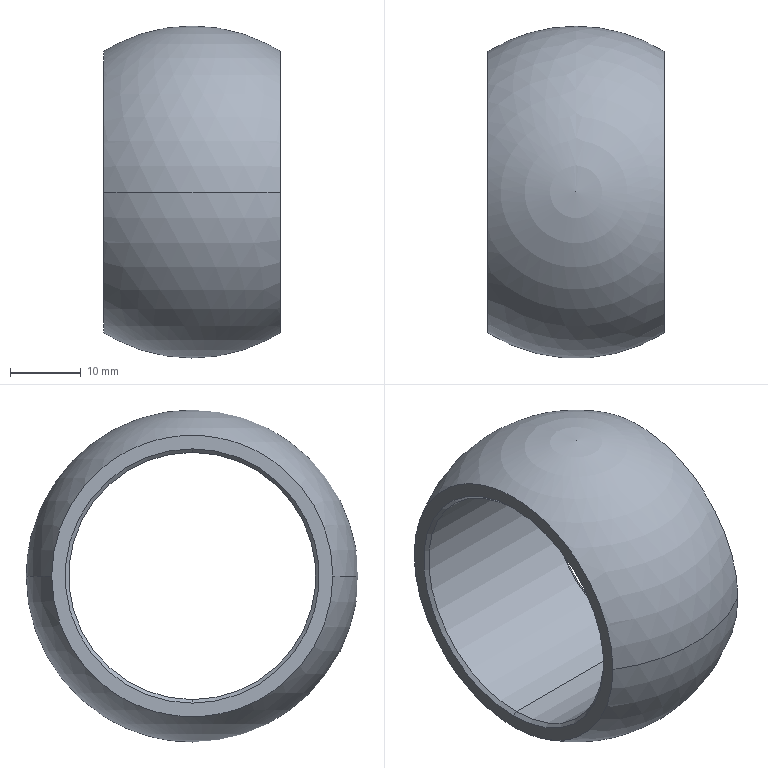Part | SolidWorks | features Chamfer 1, Revolution 1 | 1 solid | 10 faces | box 25 x 47 x 47 mm | volume 15202 mm3 | cone 4 | cylinder 2 | sphere 2 | plane 2 | commonest cylinder face diameters 35 x2
STEP:
#1=CARTESIAN_POINT('',(12.,0.,17.5));
#2=VERTEX_POINT('',#1);
#3=CARTESIAN_POINT('',(12.,0.,-17.5));
#4=VERTEX_POINT('',#3);
#5=CARTESIAN_POINT('',(12.,0.,0.));
#6=DIRECTION('',(1.,0.,0.));
#7=DIRECTION('',(0.,0.,1.));
#8=AXIS2_PLACEMENT_3D('',#5,#6,#7);
#9=CIRCLE('',#8,17.5);
#10=EDGE_CURVE('',#2,#4,#9,.T.);
#11=ORIENTED_EDGE('',*,*,#10,.F.);
#12=CARTESIAN_POINT('',(12.5,0.,18.));
#13=VERTEX_POINT('',#12);
#14=CARTESIAN_POINT('',(12.5,0.,18.));
#15=DIRECTION('',(0.7071,0.,0.7071));
#16=VECTOR('',#15,1000.);
#17=LINE('',#14,#16);
#18=EDGE_CURVE('',#2,#13,#17,.T.);
#19=ORIENTED_EDGE('',*,*,#18,.T.);
#20=CARTESIAN_POINT('',(12.5,0.,-18.));
#21=VERTEX_POINT('',#20);
#22=CARTESIAN_POINT('',(12.5,0.,0.));
#23=DIRECTION('',(-1.,0.,0.));
#24=DIRECTION('',(0.,0.,1.));
#25=AXIS2_PLACEMENT_3D('',#22,#23,#24);
#26=CIRCLE('',#25,18.);
#27=EDGE_CURVE('',#21,#13,#26,.T.);
#28=ORIENTED_EDGE('',*,*,#27,.F.);
#29=CARTESIAN_POINT('',(12.5,0.,-18.));
#30=DIRECTION('',(0.7071,0.,-0.7071));
#31=VECTOR('',#30,1000.);
#32=LINE('',#29,#31);
#33=EDGE_CURVE('',#4,#21,#32,.T.);
#34=ORIENTED_EDGE('',*,*,#33,.F.);
#35=EDGE_LOOP('',(#11,#19,#28,#34));
#36=FACE_OUTER_BOUND('',#35,.T.);
#37=CARTESIAN_POINT('',(12.5,0.,0.));
#38=DIRECTION('',(1.,0.,0.));
#39=DIRECTION('',(0.,0.,-1.));
#40=AXIS2_PLACEMENT_3D('',#37,#38,#39);
#41=CONICAL_SURFACE('',#40,18.,0.7854);
#42=ADVANCED_FACE('',(#36),#41,.F.);
#43=CARTESIAN_POINT('',(-12.,0.,-17.5));
#44=VERTEX_POINT('',#43);
#45=CARTESIAN_POINT('',(-12.,0.,17.5));
#46=VERTEX_POINT('',#45);
#47=CARTESIAN_POINT('',(-12.,0.,0.));
#48=DIRECTION('',(-1.,0.,0.));
#49=DIRECTION('',(0.,0.,-1.));
#50=AXIS2_PLACEMENT_3D('',#47,#48,#49);
#51=CIRCLE('',#50,17.5);
#52=EDGE_CURVE('',#44,#46,#51,.T.);
#53=ORIENTED_EDGE('',*,*,#52,.F.);
#54=CARTESIAN_POINT('',(-12.5,0.,-18.));
#55=VERTEX_POINT('',#54);
#56=CARTESIAN_POINT('',(-12.,0.,-17.5));
#57=DIRECTION('',(-0.7071,0.,-0.7071));
#58=VECTOR('',#57,1000.);
#59=LINE('',#56,#58);
#60=EDGE_CURVE('',#44,#55,#59,.T.);
#61=ORIENTED_EDGE('',*,*,#60,.T.);
#62=CARTESIAN_POINT('',(-12.5,0.,18.));
#63=VERTEX_POINT('',#62);
#64=CARTESIAN_POINT('',(-12.5,0.,0.));
#65=DIRECTION('',(1.,0.,0.));
#66=DIRECTION('',(0.,0.,-1.));
#67=AXIS2_PLACEMENT_3D('',#64,#65,#66);
#68=CIRCLE('',#67,18.);
#69=EDGE_CURVE('',#63,#55,#68,.T.);
#70=ORIENTED_EDGE('',*,*,#69,.F.);
#71=CARTESIAN_POINT('',(-12.,0.,17.5));
#72=DIRECTION('',(-0.7071,0.,0.7071));
#73=VECTOR('',#72,1000.);
#74=LINE('',#71,#73);
#75=EDGE_CURVE('',#46,#63,#74,.T.);
#76=ORIENTED_EDGE('',*,*,#75,.F.);
#77=EDGE_LOOP('',(#53,#61,#70,#76));
#78=FACE_OUTER_BOUND('',#77,.T.);
#79=CARTESIAN_POINT('',(-12.,0.,0.));
#80=DIRECTION('',(-1.,0.,0.));
#81=DIRECTION('',(0.,0.,1.));
#82=AXIS2_PLACEMENT_3D('',#79,#80,#81);
#83=CONICAL_SURFACE('',#82,17.5,0.7854);
#84=ADVANCED_FACE('',(#78),#83,.F.);
#85=ORIENTED_EDGE('',*,*,#10,.T.);
#86=CARTESIAN_POINT('',(-75.393,0.,-17.5));
#87=DIRECTION('',(-1.,0.,0.));
#88=VECTOR('',#87,1000.);
#89=LINE('',#86,#88);
#90=EDGE_CURVE('',#4,#44,#89,.T.);
#91=ORIENTED_EDGE('',*,*,#90,.T.);
#92=ORIENTED_EDGE('',*,*,#52,.T.);
#93=CARTESIAN_POINT('',(-75.393,0.,17.5));
#94=DIRECTION('',(-1.,0.,0.));
#95=VECTOR('',#94,1000.);
#96=LINE('',#93,#95);
#97=EDGE_CURVE('',#2,#46,#96,.T.);
#98=ORIENTED_EDGE('',*,*,#97,.F.);
#99=EDGE_LOOP('',(#85,#91,#92,#98));
#100=FACE_OUTER_BOUND('',#99,.T.);
#101=CARTESIAN_POINT('',(-75.393,0.,0.));
#102=DIRECTION('',(-1.,0.,0.));
#103=DIRECTION('',(0.,0.,1.));
#104=AXIS2_PLACEMENT_3D('',#101,#102,#103);
#105=CYLINDRICAL_SURFACE('',#104,17.5);
#106=ADVANCED_FACE('',(#100),#105,.F.);
#107=CARTESIAN_POINT('',(12.5,19.9,0.));
#108=VERTEX_POINT('',#107);
#109=CARTESIAN_POINT('',(12.5,-19.9,0.));
#110=VERTEX_POINT('',#109);
#111=CARTESIAN_POINT('',(12.5,0.,0.));
#112=DIRECTION('',(-1.,0.,0.));
#113=DIRECTION('',(0.,0.,1.));
#114=AXIS2_PLACEMENT_3D('',#111,#112,#113);
#115=CIRCLE('',#114,19.9);
#116=EDGE_CURVE('',#108,#110,#115,.T.);
#117=ORIENTED_EDGE('',*,*,#116,.T.);
#118=CARTESIAN_POINT('',(-12.5,-19.9,0.));
#119=VERTEX_POINT('',#118);
#120=CARTESIAN_POINT('',(0.,0.,0.));
#121=DIRECTION('',(0.,0.,-1.));
#122=DIRECTION('',(0.,1.,0.));
#123=AXIS2_PLACEMENT_3D('',#120,#121,#122);
#124=CIRCLE('',#123,23.5);
#125=EDGE_CURVE('',#110,#119,#124,.T.);
#126=ORIENTED_EDGE('',*,*,#125,.T.);
#127=CARTESIAN_POINT('',(-12.5,19.9,0.));
#128=VERTEX_POINT('',#127);
#129=CARTESIAN_POINT('',(-12.5,0.,0.));
#130=DIRECTION('',(-1.,0.,0.));
#131=DIRECTION('',(0.,0.,1.));
#132=AXIS2_PLACEMENT_3D('',#129,#130,#131);
#133=CIRCLE('',#132,19.9);
#134=EDGE_CURVE('',#128,#119,#133,.T.);
#135=ORIENTED_EDGE('',*,*,#134,.F.);
#136=CARTESIAN_POINT('',(0.,0.,0.));
#137=DIRECTION('',(0.,0.,1.));
#138=DIRECTION('',(1.,0.,0.));
#139=AXIS2_PLACEMENT_3D('',#136,#137,#138);
#140=CIRCLE('',#139,23.5);
#141=EDGE_CURVE('',#108,#128,#140,.T.);
#142=ORIENTED_EDGE('',*,*,#141,.F.);
#143=EDGE_LOOP('',(#117,#126,#135,#142));
#144=FACE_OUTER_BOUND('',#143,.T.);
#145=CARTESIAN_POINT('',(0.,0.,0.));
#146=DIRECTION('',(0.,0.,-1.));
#147=DIRECTION('',(0.,1.,0.));
#148=AXIS2_PLACEMENT_3D('',#145,#146,#147);
#149=SPHERICAL_SURFACE('',#148,23.5);
#150=ADVANCED_FACE('',(#144),#149,.T.);
#151=ORIENTED_EDGE('',*,*,#125,.F.);
#152=CARTESIAN_POINT('',(12.5,0.,0.));
#153=DIRECTION('',(-1.,0.,0.));
#154=DIRECTION('',(0.,0.,1.));
#155=AXIS2_PLACEMENT_3D('',#152,#153,#154);
#156=CIRCLE('',#155,19.9);
#157=EDGE_CURVE('',#110,#108,#156,.T.);
#158=ORIENTED_EDGE('',*,*,#157,.T.);
#159=ORIENTED_EDGE('',*,*,#141,.T.);
#160=CARTESIAN_POINT('',(-12.5,0.,0.));
#161=DIRECTION('',(-1.,0.,0.));
#162=DIRECTION('',(0.,0.,1.));
#163=AXIS2_PLACEMENT_3D('',#160,#161,#162);
#164=CIRCLE('',#163,19.9);
#165=EDGE_CURVE('',#119,#128,#164,.T.);
#166=ORIENTED_EDGE('',*,*,#165,.F.);
#167=EDGE_LOOP('',(#151,#158,#159,#166));
#168=FACE_OUTER_BOUND('',#167,.T.);
#169=CARTESIAN_POINT('',(0.,0.,0.));
#170=DIRECTION('',(0.,0.,-1.));
#171=DIRECTION('',(0.,1.,0.));
#172=AXIS2_PLACEMENT_3D('',#169,#170,#171);
#173=SPHERICAL_SURFACE('',#172,23.5);
#174=ADVANCED_FACE('',(#168),#173,.T.);
#175=ORIENTED_EDGE('',*,*,#69,.T.);
#176=CARTESIAN_POINT('',(-12.5,0.,0.));
#177=DIRECTION('',(1.,0.,0.));
#178=DIRECTION('',(0.,0.,-1.));
#179=AXIS2_PLACEMENT_3D('',#176,#177,#178);
#180=CIRCLE('',#179,18.);
#181=EDGE_CURVE('',#55,#63,#180,.T.);
#182=ORIENTED_EDGE('',*,*,#181,.T.);
#183=EDGE_LOOP('',(#175,#182));
#184=FACE_BOUND('',#183,.T.);
#185=ORIENTED_EDGE('',*,*,#134,.T.);
#186=ORIENTED_EDGE('',*,*,#165,.T.);
#187=EDGE_LOOP('',(#185,#186));
#188=FACE_OUTER_BOUND('',#187,.T.);
#189=CARTESIAN_POINT('',(-12.5,19.9,0.));
#190=DIRECTION('',(1.,0.,0.));
#191=DIRECTION('',(0.,0.,-1.));
#192=AXIS2_PLACEMENT_3D('',#189,#190,#191);
#193=PLANE('',#192);
#194=ADVANCED_FACE('',(#184,#188),#193,.F.);
#195=ORIENTED_EDGE('',*,*,#90,.F.);
#196=CARTESIAN_POINT('',(12.,0.,0.));
#197=DIRECTION('',(1.,0.,0.));
#198=DIRECTION('',(0.,0.,1.));
#199=AXIS2_PLACEMENT_3D('',#196,#197,#198);
#200=CIRCLE('',#199,17.5);
#201=EDGE_CURVE('',#4,#2,#200,.T.);
#202=ORIENTED_EDGE('',*,*,#201,.T.);
#203=ORIENTED_EDGE('',*,*,#97,.T.);
#204=CARTESIAN_POINT('',(-12.,0.,0.));
#205=DIRECTION('',(-1.,0.,0.));
#206=DIRECTION('',(0.,0.,-1.));
#207=AXIS2_PLACEMENT_3D('',#204,#205,#206);
#208=CIRCLE('',#207,17.5);
#209=EDGE_CURVE('',#46,#44,#208,.T.);
#210=ORIENTED_EDGE('',*,*,#209,.T.);
#211=EDGE_LOOP('',(#195,#202,#203,#210));
#212=FACE_OUTER_BOUND('',#211,.T.);
#213=CARTESIAN_POINT('',(-75.393,0.,0.));
#214=DIRECTION('',(-1.,0.,0.));
#215=DIRECTION('',(0.,0.,1.));
#216=AXIS2_PLACEMENT_3D('',#213,#214,#215);
#217=CYLINDRICAL_SURFACE('',#216,17.5);
#218=ADVANCED_FACE('',(#212),#217,.F.);
#219=ORIENTED_EDGE('',*,*,#27,.T.);
#220=CARTESIAN_POINT('',(12.5,0.,0.));
#221=DIRECTION('',(-1.,0.,0.));
#222=DIRECTION('',(0.,0.,1.));
#223=AXIS2_PLACEMENT_3D('',#220,#221,#222);
#224=CIRCLE('',#223,18.);
#225=EDGE_CURVE('',#13,#21,#224,.T.);
#226=ORIENTED_EDGE('',*,*,#225,.T.);
#227=EDGE_LOOP('',(#219,#226));
#228=FACE_BOUND('',#227,.T.);
#229=ORIENTED_EDGE('',*,*,#116,.F.);
#230=ORIENTED_EDGE('',*,*,#157,.F.);
#231=EDGE_LOOP('',(#229,#230));
#232=FACE_OUTER_BOUND('',#231,.T.);
#233=CARTESIAN_POINT('',(12.5,19.9,0.));
#234=DIRECTION('',(-1.,0.,0.));
#235=DIRECTION('',(0.,0.,1.));
#236=AXIS2_PLACEMENT_3D('',#233,#234,#235);
#237=PLANE('',#236);
#238=ADVANCED_FACE('',(#228,#232),#237,.F.);
#239=ORIENTED_EDGE('',*,*,#60,.F.);
#240=ORIENTED_EDGE('',*,*,#209,.F.);
#241=ORIENTED_EDGE('',*,*,#75,.T.);
#242=ORIENTED_EDGE('',*,*,#181,.F.);
#243=EDGE_LOOP('',(#239,#240,#241,#242));
#244=FACE_OUTER_BOUND('',#243,.T.);
#245=CARTESIAN_POINT('',(-12.,0.,0.));
#246=DIRECTION('',(-1.,0.,0.));
#247=DIRECTION('',(0.,0.,1.));
#248=AXIS2_PLACEMENT_3D('',#245,#246,#247);
#249=CONICAL_SURFACE('',#248,17.5,0.7854);
#250=ADVANCED_FACE('',(#244),#249,.F.);
#251=ORIENTED_EDGE('',*,*,#18,.F.);
#252=ORIENTED_EDGE('',*,*,#201,.F.);
#253=ORIENTED_EDGE('',*,*,#33,.T.);
#254=ORIENTED_EDGE('',*,*,#225,.F.);
#255=EDGE_LOOP('',(#251,#252,#253,#254));
#256=FACE_OUTER_BOUND('',#255,.T.);
#257=CARTESIAN_POINT('',(12.5,0.,0.));
#258=DIRECTION('',(1.,0.,0.));
#259=DIRECTION('',(0.,0.,-1.));
#260=AXIS2_PLACEMENT_3D('',#257,#258,#259);
#261=CONICAL_SURFACE('',#260,18.,0.7854);
#262=ADVANCED_FACE('',(#256),#261,.F.);
#263=CLOSED_SHELL('',(#42,#84,#106,#150,#174,#194,#218,#238,#250,#262));
#264=MANIFOLD_SOLID_BREP('',#263);
#265=CARTESIAN_POINT('',(0.,0.,0.));
#266=DIRECTION('',(0.,0.,1.));
#267=DIRECTION('',(1.,0.,0.));
#268=AXIS2_PLACEMENT_3D('',#265,#266,#267);
#269=(LENGTH_UNIT()NAMED_UNIT(*)SI_UNIT(.MILLI.,.METRE.));
#270=UNCERTAINTY_MEASURE_WITH_UNIT(LENGTH_MEASURE(0.00001),#269,'','');
#271=(NAMED_UNIT(*)PLANE_ANGLE_UNIT()SI_UNIT($,.RADIAN.));
#272=(NAMED_UNIT(*)SI_UNIT($,.STERADIAN.)SOLID_ANGLE_UNIT());
#273=(GEOMETRIC_REPRESENTATION_CONTEXT(3)GLOBAL_UNCERTAINTY_ASSIGNED_CONTEXT((#270))GLOBAL_UNIT_ASSIGNED_CONTEXT((#269,#271,#272))REPRESENTATION_CONTEXT('',''));
#274=ADVANCED_BREP_SHAPE_REPRESENTATION('',(#264,#268),#273);